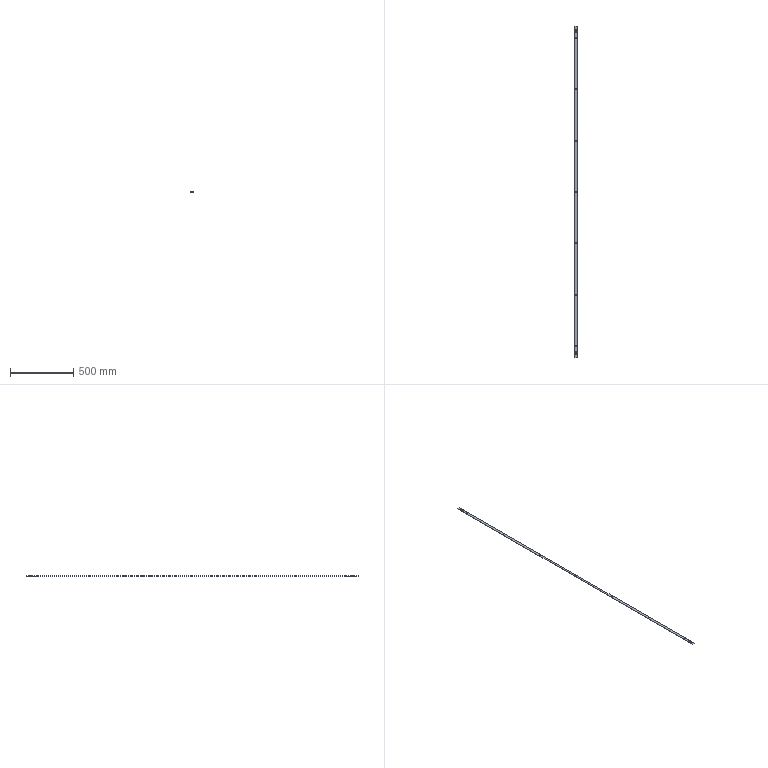Part | 1 solid | 36 faces | box 20 x 2616 x 1.5 mm | volume 77453 mm3 | cylinder 22 | plane 14 | commonest cylinder face diameters 6.2 x14 4 x8
STEP:
#1=CARTESIAN_POINT('',(-3.1,-1213.,-1.5));
#2=VERTEX_POINT('',#1);
#3=CARTESIAN_POINT('',(3.1,-1213.,-1.5));
#4=VERTEX_POINT('',#3);
#5=CARTESIAN_POINT('',(0.,-1213.,-1.5));
#6=DIRECTION('',(0.,0.,1.));
#7=DIRECTION('',(1.,0.,0.));
#8=AXIS2_PLACEMENT_3D('',#5,#6,#7);
#9=CIRCLE('',#8,3.1);
#10=EDGE_CURVE('',#2,#4,#9,.T.);
#11=ORIENTED_EDGE('',*,*,#10,.F.);
#12=CARTESIAN_POINT('',(-3.1,-1213.,0.));
#13=VERTEX_POINT('',#12);
#14=CARTESIAN_POINT('',(-3.1,-1213.,-10.));
#15=DIRECTION('',(0.,0.,1.));
#16=VECTOR('',#15,1000.);
#17=LINE('',#14,#16);
#18=EDGE_CURVE('',#2,#13,#17,.T.);
#19=ORIENTED_EDGE('',*,*,#18,.T.);
#20=CARTESIAN_POINT('',(3.1,-1213.,0.));
#21=VERTEX_POINT('',#20);
#22=CARTESIAN_POINT('',(0.,-1213.,0.));
#23=DIRECTION('',(0.,0.,1.));
#24=DIRECTION('',(-1.,0.,0.));
#25=AXIS2_PLACEMENT_3D('',#22,#23,#24);
#26=CIRCLE('',#25,3.1);
#27=EDGE_CURVE('',#13,#21,#26,.T.);
#28=ORIENTED_EDGE('',*,*,#27,.T.);
#29=CARTESIAN_POINT('',(3.1,-1213.,-10.));
#30=DIRECTION('',(0.,0.,1.));
#31=VECTOR('',#30,1000.);
#32=LINE('',#29,#31);
#33=EDGE_CURVE('',#4,#21,#32,.T.);
#34=ORIENTED_EDGE('',*,*,#33,.F.);
#35=EDGE_LOOP('',(#11,#19,#28,#34));
#36=FACE_OUTER_BOUND('',#35,.T.);
#37=CARTESIAN_POINT('',(0.,-1213.,-10.));
#38=DIRECTION('',(0.,0.,1.));
#39=DIRECTION('',(1.,0.,0.));
#40=AXIS2_PLACEMENT_3D('',#37,#38,#39);
#41=CYLINDRICAL_SURFACE('',#40,3.1);
#42=ADVANCED_FACE('',(#36),#41,.F.);
#43=CARTESIAN_POINT('',(-3.1,-808.667,-1.5));
#44=VERTEX_POINT('',#43);
#45=CARTESIAN_POINT('',(3.1,-808.667,-1.5));
#46=VERTEX_POINT('',#45);
#47=CARTESIAN_POINT('',(0.,-808.667,-1.5));
#48=DIRECTION('',(0.,0.,1.));
#49=DIRECTION('',(1.,0.,0.));
#50=AXIS2_PLACEMENT_3D('',#47,#48,#49);
#51=CIRCLE('',#50,3.1);
#52=EDGE_CURVE('',#44,#46,#51,.T.);
#53=ORIENTED_EDGE('',*,*,#52,.F.);
#54=CARTESIAN_POINT('',(-3.1,-808.667,0.));
#55=VERTEX_POINT('',#54);
#56=CARTESIAN_POINT('',(-3.1,-808.667,-10.));
#57=DIRECTION('',(0.,0.,1.));
#58=VECTOR('',#57,1000.);
#59=LINE('',#56,#58);
#60=EDGE_CURVE('',#44,#55,#59,.T.);
#61=ORIENTED_EDGE('',*,*,#60,.T.);
#62=CARTESIAN_POINT('',(3.1,-808.667,0.));
#63=VERTEX_POINT('',#62);
#64=CARTESIAN_POINT('',(0.,-808.667,0.));
#65=DIRECTION('',(0.,0.,1.));
#66=DIRECTION('',(-1.,0.,0.));
#67=AXIS2_PLACEMENT_3D('',#64,#65,#66);
#68=CIRCLE('',#67,3.1);
#69=EDGE_CURVE('',#55,#63,#68,.T.);
#70=ORIENTED_EDGE('',*,*,#69,.T.);
#71=CARTESIAN_POINT('',(3.1,-808.667,-10.));
#72=DIRECTION('',(0.,0.,1.));
#73=VECTOR('',#72,1000.);
#74=LINE('',#71,#73);
#75=EDGE_CURVE('',#46,#63,#74,.T.);
#76=ORIENTED_EDGE('',*,*,#75,.F.);
#77=EDGE_LOOP('',(#53,#61,#70,#76));
#78=FACE_OUTER_BOUND('',#77,.T.);
#79=CARTESIAN_POINT('',(0.,-808.667,-10.));
#80=DIRECTION('',(0.,0.,1.));
#81=DIRECTION('',(1.,0.,0.));
#82=AXIS2_PLACEMENT_3D('',#79,#80,#81);
#83=CYLINDRICAL_SURFACE('',#82,3.1);
#84=ADVANCED_FACE('',(#78),#83,.F.);
#85=CARTESIAN_POINT('',(-3.1,404.333,-1.5));
#86=VERTEX_POINT('',#85);
#87=CARTESIAN_POINT('',(3.1,404.333,-1.5));
#88=VERTEX_POINT('',#87);
#89=CARTESIAN_POINT('',(0.,404.333,-1.5));
#90=DIRECTION('',(0.,0.,1.));
#91=DIRECTION('',(1.,0.,0.));
#92=AXIS2_PLACEMENT_3D('',#89,#90,#91);
#93=CIRCLE('',#92,3.1);
#94=EDGE_CURVE('',#86,#88,#93,.T.);
#95=ORIENTED_EDGE('',*,*,#94,.F.);
#96=CARTESIAN_POINT('',(-3.1,404.333,0.));
#97=VERTEX_POINT('',#96);
#98=CARTESIAN_POINT('',(-3.1,404.333,-10.));
#99=DIRECTION('',(0.,0.,1.));
#100=VECTOR('',#99,1000.);
#101=LINE('',#98,#100);
#102=EDGE_CURVE('',#86,#97,#101,.T.);
#103=ORIENTED_EDGE('',*,*,#102,.T.);
#104=CARTESIAN_POINT('',(3.1,404.333,0.));
#105=VERTEX_POINT('',#104);
#106=CARTESIAN_POINT('',(0.,404.333,0.));
#107=DIRECTION('',(0.,0.,1.));
#108=DIRECTION('',(1.,0.,0.));
#109=AXIS2_PLACEMENT_3D('',#106,#107,#108);
#110=CIRCLE('',#109,3.1);
#111=EDGE_CURVE('',#97,#105,#110,.T.);
#112=ORIENTED_EDGE('',*,*,#111,.T.);
#113=CARTESIAN_POINT('',(3.1,404.333,-10.));
#114=DIRECTION('',(0.,0.,1.));
#115=VECTOR('',#114,1000.);
#116=LINE('',#113,#115);
#117=EDGE_CURVE('',#88,#105,#116,.T.);
#118=ORIENTED_EDGE('',*,*,#117,.F.);
#119=EDGE_LOOP('',(#95,#103,#112,#118));
#120=FACE_OUTER_BOUND('',#119,.T.);
#121=CARTESIAN_POINT('',(0.,404.333,-10.));
#122=DIRECTION('',(0.,0.,1.));
#123=DIRECTION('',(1.,0.,0.));
#124=AXIS2_PLACEMENT_3D('',#121,#122,#123);
#125=CYLINDRICAL_SURFACE('',#124,3.1);
#126=ADVANCED_FACE('',(#120),#125,.F.);
#127=CARTESIAN_POINT('',(-3.1,808.667,-1.5));
#128=VERTEX_POINT('',#127);
#129=CARTESIAN_POINT('',(3.1,808.667,-1.5));
#130=VERTEX_POINT('',#129);
#131=CARTESIAN_POINT('',(0.,808.667,-1.5));
#132=DIRECTION('',(0.,0.,1.));
#133=DIRECTION('',(1.,0.,0.));
#134=AXIS2_PLACEMENT_3D('',#131,#132,#133);
#135=CIRCLE('',#134,3.1);
#136=EDGE_CURVE('',#128,#130,#135,.T.);
#137=ORIENTED_EDGE('',*,*,#136,.F.);
#138=CARTESIAN_POINT('',(-3.1,808.667,0.));
#139=VERTEX_POINT('',#138);
#140=CARTESIAN_POINT('',(-3.1,808.667,-10.));
#141=DIRECTION('',(0.,0.,1.));
#142=VECTOR('',#141,1000.);
#143=LINE('',#140,#142);
#144=EDGE_CURVE('',#128,#139,#143,.T.);
#145=ORIENTED_EDGE('',*,*,#144,.T.);
#146=CARTESIAN_POINT('',(3.1,808.667,0.));
#147=VERTEX_POINT('',#146);
#148=CARTESIAN_POINT('',(0.,808.667,0.));
#149=DIRECTION('',(0.,0.,1.));
#150=DIRECTION('',(1.,0.,0.));
#151=AXIS2_PLACEMENT_3D('',#148,#149,#150);
#152=CIRCLE('',#151,3.1);
#153=EDGE_CURVE('',#139,#147,#152,.T.);
#154=ORIENTED_EDGE('',*,*,#153,.T.);
#155=CARTESIAN_POINT('',(3.1,808.667,-10.));
#156=DIRECTION('',(0.,0.,1.));
#157=VECTOR('',#156,1000.);
#158=LINE('',#155,#157);
#159=EDGE_CURVE('',#130,#147,#158,.T.);
#160=ORIENTED_EDGE('',*,*,#159,.F.);
#161=EDGE_LOOP('',(#137,#145,#154,#160));
#162=FACE_OUTER_BOUND('',#161,.T.);
#163=CARTESIAN_POINT('',(0.,808.667,-10.));
#164=DIRECTION('',(0.,0.,1.));
#165=DIRECTION('',(1.,0.,0.));
#166=AXIS2_PLACEMENT_3D('',#163,#164,#165);
#167=CYLINDRICAL_SURFACE('',#166,3.1);
#168=ADVANCED_FACE('',(#162),#167,.F.);
#169=CARTESIAN_POINT('',(-3.1,1213.,-1.5));
#170=VERTEX_POINT('',#169);
#171=CARTESIAN_POINT('',(3.1,1213.,-1.5));
#172=VERTEX_POINT('',#171);
#173=CARTESIAN_POINT('',(0.,1213.,-1.5));
#174=DIRECTION('',(0.,0.,1.));
#175=DIRECTION('',(1.,0.,0.));
#176=AXIS2_PLACEMENT_3D('',#173,#174,#175);
#177=CIRCLE('',#176,3.1);
#178=EDGE_CURVE('',#170,#172,#177,.T.);
#179=ORIENTED_EDGE('',*,*,#178,.F.);
#180=CARTESIAN_POINT('',(-3.1,1213.,0.));
#181=VERTEX_POINT('',#180);
#182=CARTESIAN_POINT('',(-3.1,1213.,-10.));
#183=DIRECTION('',(0.,0.,1.));
#184=VECTOR('',#183,1000.);
#185=LINE('',#182,#184);
#186=EDGE_CURVE('',#170,#181,#185,.T.);
#187=ORIENTED_EDGE('',*,*,#186,.T.);
#188=CARTESIAN_POINT('',(3.1,1213.,0.));
#189=VERTEX_POINT('',#188);
#190=CARTESIAN_POINT('',(0.,1213.,0.));
#191=DIRECTION('',(0.,0.,1.));
#192=DIRECTION('',(1.,0.,0.));
#193=AXIS2_PLACEMENT_3D('',#190,#191,#192);
#194=CIRCLE('',#193,3.1);
#195=EDGE_CURVE('',#181,#189,#194,.T.);
#196=ORIENTED_EDGE('',*,*,#195,.T.);
#197=CARTESIAN_POINT('',(3.1,1213.,-10.));
#198=DIRECTION('',(0.,0.,1.));
#199=VECTOR('',#198,1000.);
#200=LINE('',#197,#199);
#201=EDGE_CURVE('',#172,#189,#200,.T.);
#202=ORIENTED_EDGE('',*,*,#201,.F.);
#203=EDGE_LOOP('',(#179,#187,#196,#202));
#204=FACE_OUTER_BOUND('',#203,.T.);
#205=CARTESIAN_POINT('',(0.,1213.,-10.));
#206=DIRECTION('',(0.,0.,1.));
#207=DIRECTION('',(1.,0.,0.));
#208=AXIS2_PLACEMENT_3D('',#205,#206,#207);
#209=CYLINDRICAL_SURFACE('',#208,3.1);
#210=ADVANCED_FACE('',(#204),#209,.F.);
#211=CARTESIAN_POINT('',(-3.1,-404.333,-1.5));
#212=VERTEX_POINT('',#211);
#213=CARTESIAN_POINT('',(3.1,-404.333,-1.5));
#214=VERTEX_POINT('',#213);
#215=CARTESIAN_POINT('',(0.,-404.333,-1.5));
#216=DIRECTION('',(0.,0.,1.));
#217=DIRECTION('',(1.,0.,0.));
#218=AXIS2_PLACEMENT_3D('',#215,#216,#217);
#219=CIRCLE('',#218,3.1);
#220=EDGE_CURVE('',#212,#214,#219,.T.);
#221=ORIENTED_EDGE('',*,*,#220,.F.);
#222=CARTESIAN_POINT('',(-3.1,-404.333,0.));
#223=VERTEX_POINT('',#222);
#224=CARTESIAN_POINT('',(-3.1,-404.333,-10.));
#225=DIRECTION('',(0.,0.,1.));
#226=VECTOR('',#225,1000.);
#227=LINE('',#224,#226);
#228=EDGE_CURVE('',#212,#223,#227,.T.);
#229=ORIENTED_EDGE('',*,*,#228,.T.);
#230=CARTESIAN_POINT('',(3.1,-404.333,0.));
#231=VERTEX_POINT('',#230);
#232=CARTESIAN_POINT('',(0.,-404.333,0.));
#233=DIRECTION('',(0.,0.,1.));
#234=DIRECTION('',(-1.,0.,0.));
#235=AXIS2_PLACEMENT_3D('',#232,#233,#234);
#236=CIRCLE('',#235,3.1);
#237=EDGE_CURVE('',#223,#231,#236,.T.);
#238=ORIENTED_EDGE('',*,*,#237,.T.);
#239=CARTESIAN_POINT('',(3.1,-404.333,-10.));
#240=DIRECTION('',(0.,0.,1.));
#241=VECTOR('',#240,1000.);
#242=LINE('',#239,#241);
#243=EDGE_CURVE('',#214,#231,#242,.T.);
#244=ORIENTED_EDGE('',*,*,#243,.F.);
#245=EDGE_LOOP('',(#221,#229,#238,#244));
#246=FACE_OUTER_BOUND('',#245,.T.);
#247=CARTESIAN_POINT('',(0.,-404.333,-10.));
#248=DIRECTION('',(0.,0.,1.));
#249=DIRECTION('',(1.,0.,0.));
#250=AXIS2_PLACEMENT_3D('',#247,#248,#249);
#251=CYLINDRICAL_SURFACE('',#250,3.1);
#252=ADVANCED_FACE('',(#246),#251,.F.);
#253=CARTESIAN_POINT('',(-3.1,0.,-1.5));
#254=VERTEX_POINT('',#253);
#255=CARTESIAN_POINT('',(3.1,0.,-1.5));
#256=VERTEX_POINT('',#255);
#257=CARTESIAN_POINT('',(0.,0.,-1.5));
#258=DIRECTION('',(0.,0.,1.));
#259=DIRECTION('',(1.,0.,0.));
#260=AXIS2_PLACEMENT_3D('',#257,#258,#259);
#261=CIRCLE('',#260,3.1);
#262=EDGE_CURVE('',#254,#256,#261,.T.);
#263=ORIENTED_EDGE('',*,*,#262,.F.);
#264=CARTESIAN_POINT('',(-3.1,0.,0.));
#265=VERTEX_POINT('',#264);
#266=CARTESIAN_POINT('',(-3.1,0.,-10.));
#267=DIRECTION('',(0.,0.,1.));
#268=VECTOR('',#267,1000.);
#269=LINE('',#266,#268);
#270=EDGE_CURVE('',#254,#265,#269,.T.);
#271=ORIENTED_EDGE('',*,*,#270,.T.);
#272=CARTESIAN_POINT('',(3.1,0.,0.));
#273=VERTEX_POINT('',#272);
#274=CARTESIAN_POINT('',(0.,0.,0.));
#275=DIRECTION('',(0.,0.,1.));
#276=DIRECTION('',(1.,0.,0.));
#277=AXIS2_PLACEMENT_3D('',#274,#275,#276);
#278=CIRCLE('',#277,3.1);
#279=EDGE_CURVE('',#265,#273,#278,.T.);
#280=ORIENTED_EDGE('',*,*,#279,.T.);
#281=CARTESIAN_POINT('',(3.1,0.,-10.));
#282=DIRECTION('',(0.,0.,1.));
#283=VECTOR('',#282,1000.);
#284=LINE('',#281,#283);
#285=EDGE_CURVE('',#256,#273,#284,.T.);
#286=ORIENTED_EDGE('',*,*,#285,.F.);
#287=EDGE_LOOP('',(#263,#271,#280,#286));
#288=FACE_OUTER_BOUND('',#287,.T.);
#289=CARTESIAN_POINT('',(0.,0.,-10.));
#290=DIRECTION('',(0.,0.,1.));
#291=DIRECTION('',(1.,0.,0.));
#292=AXIS2_PLACEMENT_3D('',#289,#290,#291);
#293=CYLINDRICAL_SURFACE('',#292,3.1);
#294=ADVANCED_FACE('',(#288),#293,.F.);
#295=CARTESIAN_POINT('',(10.,-1308.,0.));
#296=VERTEX_POINT('',#295);
#297=CARTESIAN_POINT('',(10.,1308.,0.));
#298=VERTEX_POINT('',#297);
#299=CARTESIAN_POINT('',(10.,1308.,0.));
#300=DIRECTION('',(0.,1.,0.));
#301=VECTOR('',#300,1000.);
#302=LINE('',#299,#301);
#303=EDGE_CURVE('',#296,#298,#302,.T.);
#304=ORIENTED_EDGE('',*,*,#303,.F.);
#305=CARTESIAN_POINT('',(10.,-1308.,-1.5));
#306=VERTEX_POINT('',#305);
#307=CARTESIAN_POINT('',(10.,-1308.,-1.5));
#308=DIRECTION('',(0.,0.,1.));
#309=VECTOR('',#308,1000.);
#310=LINE('',#307,#309);
#311=EDGE_CURVE('',#306,#296,#310,.T.);
#312=ORIENTED_EDGE('',*,*,#311,.F.);
#313=CARTESIAN_POINT('',(10.,1308.,-1.5));
#314=VERTEX_POINT('',#313);
#315=CARTESIAN_POINT('',(10.,1308.,-1.5));
#316=DIRECTION('',(0.,1.,0.));
#317=VECTOR('',#316,1000.);
#318=LINE('',#315,#317);
#319=EDGE_CURVE('',#306,#314,#318,.T.);
#320=ORIENTED_EDGE('',*,*,#319,.T.);
#321=CARTESIAN_POINT('',(10.,1308.,-1.5));
#322=DIRECTION('',(0.,0.,1.));
#323=VECTOR('',#322,1000.);
#324=LINE('',#321,#323);
#325=EDGE_CURVE('',#314,#298,#324,.T.);
#326=ORIENTED_EDGE('',*,*,#325,.T.);
#327=EDGE_LOOP('',(#304,#312,#320,#326));
#328=FACE_OUTER_BOUND('',#327,.T.);
#329=CARTESIAN_POINT('',(10.,1308.,-1.5));
#330=DIRECTION('',(1.,0.,0.));
#331=DIRECTION('',(0.,1.,0.));
#332=AXIS2_PLACEMENT_3D('',#329,#330,#331);
#333=PLANE('',#332);
#334=ADVANCED_FACE('',(#328),#333,.T.);
#335=CARTESIAN_POINT('',(-10.,-1308.,0.));
#336=VERTEX_POINT('',#335);
#337=CARTESIAN_POINT('',(-10.,-1308.,0.));
#338=DIRECTION('',(1.,0.,0.));
#339=VECTOR('',#338,1000.);
#340=LINE('',#337,#339);
#341=EDGE_CURVE('',#336,#296,#340,.T.);
#342=ORIENTED_EDGE('',*,*,#341,.F.);
#343=CARTESIAN_POINT('',(-10.,-1308.,-1.5));
#344=VERTEX_POINT('',#343);
#345=CARTESIAN_POINT('',(-10.,-1308.,-1.5));
#346=DIRECTION('',(0.,0.,1.));
#347=VECTOR('',#346,1000.);
#348=LINE('',#345,#347);
#349=EDGE_CURVE('',#344,#336,#348,.T.);
#350=ORIENTED_EDGE('',*,*,#349,.F.);
#351=CARTESIAN_POINT('',(-10.,-1308.,-1.5));
#352=DIRECTION('',(1.,0.,0.));
#353=VECTOR('',#352,1000.);
#354=LINE('',#351,#353);
#355=EDGE_CURVE('',#344,#306,#354,.T.);
#356=ORIENTED_EDGE('',*,*,#355,.T.);
#357=ORIENTED_EDGE('',*,*,#311,.T.);
#358=EDGE_LOOP('',(#342,#350,#356,#357));
#359=FACE_OUTER_BOUND('',#358,.T.);
#360=CARTESIAN_POINT('',(-10.,-1308.,-1.5));
#361=DIRECTION('',(0.,-1.,0.));
#362=DIRECTION('',(0.,0.,-1.));
#363=AXIS2_PLACEMENT_3D('',#360,#361,#362);
#364=PLANE('',#363);
#365=ADVANCED_FACE('',(#359),#364,.T.);
#366=CARTESIAN_POINT('',(-10.,1308.,0.));
#367=VERTEX_POINT('',#366);
#368=CARTESIAN_POINT('',(-10.,1308.,0.));
#369=DIRECTION('',(0.,-1.,0.));
#370=VECTOR('',#369,1000.);
#371=LINE('',#368,#370);
#372=EDGE_CURVE('',#367,#336,#371,.T.);
#373=ORIENTED_EDGE('',*,*,#372,.F.);
#374=CARTESIAN_POINT('',(-10.,1308.,-1.5));
#375=VERTEX_POINT('',#374);
#376=CARTESIAN_POINT('',(-10.,1308.,-1.5));
#377=DIRECTION('',(0.,0.,1.));
#378=VECTOR('',#377,1000.);
#379=LINE('',#376,#378);
#380=EDGE_CURVE('',#375,#367,#379,.T.);
#381=ORIENTED_EDGE('',*,*,#380,.F.);
#382=CARTESIAN_POINT('',(-10.,1308.,-1.5));
#383=DIRECTION('',(0.,-1.,0.));
#384=VECTOR('',#383,1000.);
#385=LINE('',#382,#384);
#386=EDGE_CURVE('',#375,#344,#385,.T.);
#387=ORIENTED_EDGE('',*,*,#386,.T.);
#388=ORIENTED_EDGE('',*,*,#349,.T.);
#389=EDGE_LOOP('',(#373,#381,#387,#388));
#390=FACE_OUTER_BOUND('',#389,.T.);
#391=CARTESIAN_POINT('',(-10.,1308.,-1.5));
#392=DIRECTION('',(-1.,0.,0.));
#393=DIRECTION('',(0.,-1.,0.));
#394=AXIS2_PLACEMENT_3D('',#391,#392,#393);
#395=PLANE('',#394);
#396=ADVANCED_FACE('',(#390),#395,.T.);
#397=CARTESIAN_POINT('',(-10.,1308.,0.));
#398=DIRECTION('',(-1.,0.,0.));
#399=VECTOR('',#398,1000.);
#400=LINE('',#397,#399);
#401=EDGE_CURVE('',#298,#367,#400,.T.);
#402=ORIENTED_EDGE('',*,*,#401,.F.);
#403=ORIENTED_EDGE('',*,*,#325,.F.);
#404=CARTESIAN_POINT('',(-10.,1308.,-1.5));
#405=DIRECTION('',(-1.,0.,0.));
#406=VECTOR('',#405,1000.);
#407=LINE('',#404,#406);
#408=EDGE_CURVE('',#314,#375,#407,.T.);
#409=ORIENTED_EDGE('',*,*,#408,.T.);
#410=ORIENTED_EDGE('',*,*,#380,.T.);
#411=EDGE_LOOP('',(#402,#403,#409,#410));
#412=FACE_OUTER_BOUND('',#411,.T.);
#413=CARTESIAN_POINT('',(-10.,1308.,-1.5));
#414=DIRECTION('',(0.,1.,0.));
#415=DIRECTION('',(0.,0.,1.));
#416=AXIS2_PLACEMENT_3D('',#413,#414,#415);
#417=PLANE('',#416);
#418=ADVANCED_FACE('',(#412),#417,.T.);
#419=CARTESIAN_POINT('',(-4.,-1255.,-1.5));
#420=VERTEX_POINT('',#419);
#421=CARTESIAN_POINT('',(-4.,-1281.,-1.5));
#422=VERTEX_POINT('',#421);
#423=CARTESIAN_POINT('',(-4.,0.,-1.5));
#424=DIRECTION('',(0.,-1.,0.));
#425=VECTOR('',#424,1000.);
#426=LINE('',#423,#425);
#427=EDGE_CURVE('',#420,#422,#426,.T.);
#428=ORIENTED_EDGE('',*,*,#427,.T.);
#429=CARTESIAN_POINT('',(-2.,-1283.,-1.5));
#430=VERTEX_POINT('',#429);
#431=CARTESIAN_POINT('',(-2.,-1281.,-1.5));
#432=DIRECTION('',(0.,0.,1.));
#433=DIRECTION('',(1.,0.,0.));
#434=AXIS2_PLACEMENT_3D('',#431,#432,#433);
#435=CIRCLE('',#434,2.);
#436=EDGE_CURVE('',#422,#430,#435,.T.);
#437=ORIENTED_EDGE('',*,*,#436,.T.);
#438=CARTESIAN_POINT('',(2.,-1283.,-1.5));
#439=VERTEX_POINT('',#438);
#440=CARTESIAN_POINT('',(0.,-1283.,-1.5));
#441=DIRECTION('',(1.,0.,0.));
#442=VECTOR('',#441,1000.);
#443=LINE('',#440,#442);
#444=EDGE_CURVE('',#430,#439,#443,.T.);
#445=ORIENTED_EDGE('',*,*,#444,.T.);
#446=CARTESIAN_POINT('',(4.,-1281.,-1.5));
#447=VERTEX_POINT('',#446);
#448=CARTESIAN_POINT('',(2.,-1281.,-1.5));
#449=DIRECTION('',(0.,0.,1.));
#450=DIRECTION('',(1.,0.,0.));
#451=AXIS2_PLACEMENT_3D('',#448,#449,#450);
#452=CIRCLE('',#451,2.);
#453=EDGE_CURVE('',#439,#447,#452,.T.);
#454=ORIENTED_EDGE('',*,*,#453,.T.);
#455=CARTESIAN_POINT('',(4.,-1255.,-1.5));
#456=VERTEX_POINT('',#455);
#457=CARTESIAN_POINT('',(4.,0.,-1.5));
#458=DIRECTION('',(0.,1.,0.));
#459=VECTOR('',#458,1000.);
#460=LINE('',#457,#459);
#461=EDGE_CURVE('',#447,#456,#460,.T.);
#462=ORIENTED_EDGE('',*,*,#461,.T.);
#463=CARTESIAN_POINT('',(2.,-1253.,-1.5));
#464=VERTEX_POINT('',#463);
#465=CARTESIAN_POINT('',(2.,-1255.,-1.5));
#466=DIRECTION('',(0.,0.,1.));
#467=DIRECTION('',(1.,0.,0.));
#468=AXIS2_PLACEMENT_3D('',#465,#466,#467);
#469=CIRCLE('',#468,2.);
#470=EDGE_CURVE('',#456,#464,#469,.T.);
#471=ORIENTED_EDGE('',*,*,#470,.T.);
#472=CARTESIAN_POINT('',(-2.,-1253.,-1.5));
#473=VERTEX_POINT('',#472);
#474=CARTESIAN_POINT('',(0.,-1253.,-1.5));
#475=DIRECTION('',(-1.,0.,0.));
#476=VECTOR('',#475,1000.);
#477=LINE('',#474,#476);
#478=EDGE_CURVE('',#464,#473,#477,.T.);
#479=ORIENTED_EDGE('',*,*,#478,.T.);
#480=CARTESIAN_POINT('',(-2.,-1255.,-1.5));
#481=DIRECTION('',(0.,0.,1.));
#482=DIRECTION('',(1.,0.,0.));
#483=AXIS2_PLACEMENT_3D('',#480,#481,#482);
#484=CIRCLE('',#483,2.);
#485=EDGE_CURVE('',#473,#420,#484,.T.);
#486=ORIENTED_EDGE('',*,*,#485,.T.);
#487=EDGE_LOOP('',(#428,#437,#445,#454,#462,#471,#479,#486));
#488=FACE_BOUND('',#487,.T.);
#489=CARTESIAN_POINT('',(4.,1255.,-1.5));
#490=VERTEX_POINT('',#489);
#491=CARTESIAN_POINT('',(4.,1281.,-1.5));
#492=VERTEX_POINT('',#491);
#493=CARTESIAN_POINT('',(4.,0.,-1.5));
#494=DIRECTION('',(0.,1.,0.));
#495=VECTOR('',#494,1000.);
#496=LINE('',#493,#495);
#497=EDGE_CURVE('',#490,#492,#496,.T.);
#498=ORIENTED_EDGE('',*,*,#497,.T.);
#499=CARTESIAN_POINT('',(2.,1283.,-1.5));
#500=VERTEX_POINT('',#499);
#501=CARTESIAN_POINT('',(2.,1281.,-1.5));
#502=DIRECTION('',(0.,0.,1.));
#503=DIRECTION('',(1.,0.,0.));
#504=AXIS2_PLACEMENT_3D('',#501,#502,#503);
#505=CIRCLE('',#504,2.);
#506=EDGE_CURVE('',#492,#500,#505,.T.);
#507=ORIENTED_EDGE('',*,*,#506,.T.);
#508=CARTESIAN_POINT('',(-2.,1283.,-1.5));
#509=VERTEX_POINT('',#508);
#510=CARTESIAN_POINT('',(0.,1283.,-1.5));
#511=DIRECTION('',(-1.,0.,0.));
#512=VECTOR('',#511,1000.);
#513=LINE('',#510,#512);
#514=EDGE_CURVE('',#500,#509,#513,.T.);
#515=ORIENTED_EDGE('',*,*,#514,.T.);
#516=CARTESIAN_POINT('',(-4.,1281.,-1.5));
#517=VERTEX_POINT('',#516);
#518=CARTESIAN_POINT('',(-2.,1281.,-1.5));
#519=DIRECTION('',(0.,0.,1.));
#520=DIRECTION('',(1.,0.,0.));
#521=AXIS2_PLACEMENT_3D('',#518,#519,#520);
#522=CIRCLE('',#521,2.);
#523=EDGE_CURVE('',#509,#517,#522,.T.);
#524=ORIENTED_EDGE('',*,*,#523,.T.);
#525=CARTESIAN_POINT('',(-4.,1255.,-1.5));
#526=VERTEX_POINT('',#525);
#527=CARTESIAN_POINT('',(-4.,0.,-1.5));
#528=DIRECTION('',(0.,-1.,0.));
#529=VECTOR('',#528,1000.);
#530=LINE('',#527,#529);
#531=EDGE_CURVE('',#517,#526,#530,.T.);
#532=ORIENTED_EDGE('',*,*,#531,.T.);
#533=CARTESIAN_POINT('',(-2.,1253.,-1.5));
#534=VERTEX_POINT('',#533);
#535=CARTESIAN_POINT('',(-2.,1255.,-1.5));
#536=DIRECTION('',(0.,0.,1.));
#537=DIRECTION('',(1.,0.,0.));
#538=AXIS2_PLACEMENT_3D('',#535,#536,#537);
#539=CIRCLE('',#538,2.);
#540=EDGE_CURVE('',#526,#534,#539,.T.);
#541=ORIENTED_EDGE('',*,*,#540,.T.);
#542=CARTESIAN_POINT('',(2.,1253.,-1.5));
#543=VERTEX_POINT('',#542);
#544=CARTESIAN_POINT('',(0.,1253.,-1.5));
#545=DIRECTION('',(1.,0.,0.));
#546=VECTOR('',#545,1000.);
#547=LINE('',#544,#546);
#548=EDGE_CURVE('',#534,#543,#547,.T.);
#549=ORIENTED_EDGE('',*,*,#548,.T.);
#550=CARTESIAN_POINT('',(2.,1255.,-1.5));
#551=DIRECTION('',(0.,0.,1.));
#552=DIRECTION('',(1.,0.,0.));
#553=AXIS2_PLACEMENT_3D('',#550,#551,#552);
#554=CIRCLE('',#553,2.);
#555=EDGE_CURVE('',#543,#490,#554,.T.);
#556=ORIENTED_EDGE('',*,*,#555,.T.);
#557=EDGE_LOOP('',(#498,#507,#515,#524,#532,#541,#549,#556));
#558=FACE_BOUND('',#557,.T.);
#559=CARTESIAN_POINT('',(0.,-1213.,-1.5));
#560=DIRECTION('',(0.,0.,1.));
#561=DIRECTION('',(1.,0.,0.));
#562=AXIS2_PLACEMENT_3D('',#559,#560,#561);
#563=CIRCLE('',#562,3.1);
#564=EDGE_CURVE('',#4,#2,#563,.T.);
#565=ORIENTED_EDGE('',*,*,#564,.T.);
#566=ORIENTED_EDGE('',*,*,#10,.T.);
#567=EDGE_LOOP('',(#565,#566));
#568=FACE_BOUND('',#567,.T.);
#569=CARTESIAN_POINT('',(0.,-808.667,-1.5));
#570=DIRECTION('',(0.,0.,1.));
#571=DIRECTION('',(1.,0.,0.));
#572=AXIS2_PLACEMENT_3D('',#569,#570,#571);
#573=CIRCLE('',#572,3.1);
#574=EDGE_CURVE('',#46,#44,#573,.T.);
#575=ORIENTED_EDGE('',*,*,#574,.T.);
#576=ORIENTED_EDGE('',*,*,#52,.T.);
#577=EDGE_LOOP('',(#575,#576));
#578=FACE_BOUND('',#577,.T.);
#579=CARTESIAN_POINT('',(0.,404.333,-1.5));
#580=DIRECTION('',(0.,0.,1.));
#581=DIRECTION('',(1.,0.,0.));
#582=AXIS2_PLACEMENT_3D('',#579,#580,#581);
#583=CIRCLE('',#582,3.1);
#584=EDGE_CURVE('',#88,#86,#583,.T.);
#585=ORIENTED_EDGE('',*,*,#584,.T.);
#586=ORIENTED_EDGE('',*,*,#94,.T.);
#587=EDGE_LOOP('',(#585,#586));
#588=FACE_BOUND('',#587,.T.);
#589=CARTESIAN_POINT('',(0.,808.667,-1.5));
#590=DIRECTION('',(0.,0.,1.));
#591=DIRECTION('',(1.,0.,0.));
#592=AXIS2_PLACEMENT_3D('',#589,#590,#591);
#593=CIRCLE('',#592,3.1);
#594=EDGE_CURVE('',#130,#128,#593,.T.);
#595=ORIENTED_EDGE('',*,*,#594,.T.);
#596=ORIENTED_EDGE('',*,*,#136,.T.);
#597=EDGE_LOOP('',(#595,#596));
#598=FACE_BOUND('',#597,.T.);
#599=CARTESIAN_POINT('',(0.,1213.,-1.5));
#600=DIRECTION('',(0.,0.,1.));
#601=DIRECTION('',(1.,0.,0.));
#602=AXIS2_PLACEMENT_3D('',#599,#600,#601);
#603=CIRCLE('',#602,3.1);
#604=EDGE_CURVE('',#172,#170,#603,.T.);
#605=ORIENTED_EDGE('',*,*,#604,.T.);
#606=ORIENTED_EDGE('',*,*,#178,.T.);
#607=EDGE_LOOP('',(#605,#606));
#608=FACE_BOUND('',#607,.T.);
#609=CARTESIAN_POINT('',(0.,-404.333,-1.5));
#610=DIRECTION('',(0.,0.,1.));
#611=DIRECTION('',(1.,0.,0.));
#612=AXIS2_PLACEMENT_3D('',#609,#610,#611);
#613=CIRCLE('',#612,3.1);
#614=EDGE_CURVE('',#214,#212,#613,.T.);
#615=ORIENTED_EDGE('',*,*,#614,.T.);
#616=ORIENTED_EDGE('',*,*,#220,.T.);
#617=EDGE_LOOP('',(#615,#616));
#618=FACE_BOUND('',#617,.T.);
#619=CARTESIAN_POINT('',(0.,0.,-1.5));
#620=DIRECTION('',(0.,0.,1.));
#621=DIRECTION('',(1.,0.,0.));
#622=AXIS2_PLACEMENT_3D('',#619,#620,#621);
#623=CIRCLE('',#622,3.1);
#624=EDGE_CURVE('',#256,#254,#623,.T.);
#625=ORIENTED_EDGE('',*,*,#624,.T.);
#626=ORIENTED_EDGE('',*,*,#262,.T.);
#627=EDGE_LOOP('',(#625,#626));
#628=FACE_BOUND('',#627,.T.);
#629=ORIENTED_EDGE('',*,*,#319,.F.);
#630=ORIENTED_EDGE('',*,*,#355,.F.);
#631=ORIENTED_EDGE('',*,*,#386,.F.);
#632=ORIENTED_EDGE('',*,*,#408,.F.);
#633=EDGE_LOOP('',(#629,#630,#631,#632));
#634=FACE_OUTER_BOUND('',#633,.T.);
#635=CARTESIAN_POINT('',(0.,0.,-1.5));
#636=DIRECTION('',(0.,0.,1.));
#637=DIRECTION('',(1.,0.,0.));
#638=AXIS2_PLACEMENT_3D('',#635,#636,#637);
#639=PLANE('',#638);
#640=ADVANCED_FACE('',(#488,#558,#568,#578,#588,#598,#608,#618,#628,#634),#639,.F.);
#641=CARTESIAN_POINT('',(4.,-1281.,0.));
#642=VERTEX_POINT('',#641);
#643=CARTESIAN_POINT('',(4.,-1255.,0.));
#644=VERTEX_POINT('',#643);
#645=CARTESIAN_POINT('',(4.,-1253.,0.));
#646=DIRECTION('',(0.,1.,0.));
#647=VECTOR('',#646,1000.);
#648=LINE('',#645,#647);
#649=EDGE_CURVE('',#642,#644,#648,.T.);
#650=ORIENTED_EDGE('',*,*,#649,.F.);
#651=CARTESIAN_POINT('',(2.,-1283.,0.));
#652=VERTEX_POINT('',#651);
#653=CARTESIAN_POINT('',(2.,-1281.,0.));
#654=DIRECTION('',(0.,0.,-1.));
#655=DIRECTION('',(1.,0.,0.));
#656=AXIS2_PLACEMENT_3D('',#653,#654,#655);
#657=CIRCLE('',#656,2.);
#658=EDGE_CURVE('',#642,#652,#657,.T.);
#659=ORIENTED_EDGE('',*,*,#658,.T.);
#660=CARTESIAN_POINT('',(-2.,-1283.,0.));
#661=VERTEX_POINT('',#660);
#662=CARTESIAN_POINT('',(-4.,-1283.,0.));
#663=DIRECTION('',(1.,0.,0.));
#664=VECTOR('',#663,1000.);
#665=LINE('',#662,#664);
#666=EDGE_CURVE('',#661,#652,#665,.T.);
#667=ORIENTED_EDGE('',*,*,#666,.F.);
#668=CARTESIAN_POINT('',(-4.,-1281.,0.));
#669=VERTEX_POINT('',#668);
#670=CARTESIAN_POINT('',(-2.,-1281.,0.));
#671=DIRECTION('',(0.,0.,-1.));
#672=DIRECTION('',(1.,0.,0.));
#673=AXIS2_PLACEMENT_3D('',#670,#671,#672);
#674=CIRCLE('',#673,2.);
#675=EDGE_CURVE('',#661,#669,#674,.T.);
#676=ORIENTED_EDGE('',*,*,#675,.T.);
#677=CARTESIAN_POINT('',(-4.,-1255.,0.));
#678=VERTEX_POINT('',#677);
#679=CARTESIAN_POINT('',(-4.,-1253.,0.));
#680=DIRECTION('',(0.,-1.,0.));
#681=VECTOR('',#680,1000.);
#682=LINE('',#679,#681);
#683=EDGE_CURVE('',#678,#669,#682,.T.);
#684=ORIENTED_EDGE('',*,*,#683,.F.);
#685=CARTESIAN_POINT('',(-2.,-1253.,0.));
#686=VERTEX_POINT('',#685);
#687=CARTESIAN_POINT('',(-2.,-1255.,0.));
#688=DIRECTION('',(0.,0.,-1.));
#689=DIRECTION('',(1.,0.,0.));
#690=AXIS2_PLACEMENT_3D('',#687,#688,#689);
#691=CIRCLE('',#690,2.);
#692=EDGE_CURVE('',#678,#686,#691,.T.);
#693=ORIENTED_EDGE('',*,*,#692,.T.);
#694=CARTESIAN_POINT('',(2.,-1253.,0.));
#695=VERTEX_POINT('',#694);
#696=CARTESIAN_POINT('',(-4.,-1253.,0.));
#697=DIRECTION('',(-1.,0.,0.));
#698=VECTOR('',#697,1000.);
#699=LINE('',#696,#698);
#700=EDGE_CURVE('',#695,#686,#699,.T.);
#701=ORIENTED_EDGE('',*,*,#700,.F.);
#702=CARTESIAN_POINT('',(2.,-1255.,0.));
#703=DIRECTION('',(0.,0.,-1.));
#704=DIRECTION('',(1.,0.,0.));
#705=AXIS2_PLACEMENT_3D('',#702,#703,#704);
#706=CIRCLE('',#705,2.);
#707=EDGE_CURVE('',#695,#644,#706,.T.);
#708=ORIENTED_EDGE('',*,*,#707,.T.);
#709=EDGE_LOOP('',(#650,#659,#667,#676,#684,#693,#701,#708));
#710=FACE_BOUND('',#709,.T.);
#711=CARTESIAN_POINT('',(-4.,1281.,0.));
#712=VERTEX_POINT('',#711);
#713=CARTESIAN_POINT('',(-4.,1255.,0.));
#714=VERTEX_POINT('',#713);
#715=CARTESIAN_POINT('',(-4.,1253.,0.));
#716=DIRECTION('',(0.,-1.,0.));
#717=VECTOR('',#716,1000.);
#718=LINE('',#715,#717);
#719=EDGE_CURVE('',#712,#714,#718,.T.);
#720=ORIENTED_EDGE('',*,*,#719,.F.);
#721=CARTESIAN_POINT('',(-2.,1283.,0.));
#722=VERTEX_POINT('',#721);
#723=CARTESIAN_POINT('',(-2.,1281.,0.));
#724=DIRECTION('',(0.,0.,-1.));
#725=DIRECTION('',(1.,0.,0.));
#726=AXIS2_PLACEMENT_3D('',#723,#724,#725);
#727=CIRCLE('',#726,2.);
#728=EDGE_CURVE('',#712,#722,#727,.T.);
#729=ORIENTED_EDGE('',*,*,#728,.T.);
#730=CARTESIAN_POINT('',(2.,1283.,0.));
#731=VERTEX_POINT('',#730);
#732=CARTESIAN_POINT('',(-4.,1283.,0.));
#733=DIRECTION('',(-1.,0.,0.));
#734=VECTOR('',#733,1000.);
#735=LINE('',#732,#734);
#736=EDGE_CURVE('',#731,#722,#735,.T.);
#737=ORIENTED_EDGE('',*,*,#736,.F.);
#738=CARTESIAN_POINT('',(4.,1281.,0.));
#739=VERTEX_POINT('',#738);
#740=CARTESIAN_POINT('',(2.,1281.,0.));
#741=DIRECTION('',(0.,0.,-1.));
#742=DIRECTION('',(1.,0.,0.));
#743=AXIS2_PLACEMENT_3D('',#740,#741,#742);
#744=CIRCLE('',#743,2.);
#745=EDGE_CURVE('',#731,#739,#744,.T.);
#746=ORIENTED_EDGE('',*,*,#745,.T.);
#747=CARTESIAN_POINT('',(4.,1255.,0.));
#748=VERTEX_POINT('',#747);
#749=CARTESIAN_POINT('',(4.,1253.,0.));
#750=DIRECTION('',(0.,1.,0.));
#751=VECTOR('',#750,1000.);
#752=LINE('',#749,#751);
#753=EDGE_CURVE('',#748,#739,#752,.T.);
#754=ORIENTED_EDGE('',*,*,#753,.F.);
#755=CARTESIAN_POINT('',(2.,1253.,0.));
#756=VERTEX_POINT('',#755);
#757=CARTESIAN_POINT('',(2.,1255.,0.));
#758=DIRECTION('',(0.,0.,-1.));
#759=DIRECTION('',(1.,0.,0.));
#760=AXIS2_PLACEMENT_3D('',#757,#758,#759);
#761=CIRCLE('',#760,2.);
#762=EDGE_CURVE('',#748,#756,#761,.T.);
#763=ORIENTED_EDGE('',*,*,#762,.T.);
#764=CARTESIAN_POINT('',(-2.,1253.,0.));
#765=VERTEX_POINT('',#764);
#766=CARTESIAN_POINT('',(-4.,1253.,0.));
#767=DIRECTION('',(1.,0.,0.));
#768=VECTOR('',#767,1000.);
#769=LINE('',#766,#768);
#770=EDGE_CURVE('',#765,#756,#769,.T.);
#771=ORIENTED_EDGE('',*,*,#770,.F.);
#772=CARTESIAN_POINT('',(-2.,1255.,0.));
#773=DIRECTION('',(0.,0.,-1.));
#774=DIRECTION('',(1.,0.,0.));
#775=AXIS2_PLACEMENT_3D('',#772,#773,#774);
#776=CIRCLE('',#775,2.);
#777=EDGE_CURVE('',#765,#714,#776,.T.);
#778=ORIENTED_EDGE('',*,*,#777,.T.);
#779=EDGE_LOOP('',(#720,#729,#737,#746,#754,#763,#771,#778));
#780=FACE_BOUND('',#779,.T.);
#781=CARTESIAN_POINT('',(0.,-1213.,0.));
#782=DIRECTION('',(0.,0.,1.));
#783=DIRECTION('',(-1.,0.,0.));
#784=AXIS2_PLACEMENT_3D('',#781,#782,#783);
#785=CIRCLE('',#784,3.1);
#786=EDGE_CURVE('',#21,#13,#785,.T.);
#787=ORIENTED_EDGE('',*,*,#786,.F.);
#788=ORIENTED_EDGE('',*,*,#27,.F.);
#789=EDGE_LOOP('',(#787,#788));
#790=FACE_BOUND('',#789,.T.);
#791=CARTESIAN_POINT('',(0.,-808.667,0.));
#792=DIRECTION('',(0.,0.,1.));
#793=DIRECTION('',(-1.,0.,0.));
#794=AXIS2_PLACEMENT_3D('',#791,#792,#793);
#795=CIRCLE('',#794,3.1);
#796=EDGE_CURVE('',#63,#55,#795,.T.);
#797=ORIENTED_EDGE('',*,*,#796,.F.);
#798=ORIENTED_EDGE('',*,*,#69,.F.);
#799=EDGE_LOOP('',(#797,#798));
#800=FACE_BOUND('',#799,.T.);
#801=CARTESIAN_POINT('',(0.,404.333,0.));
#802=DIRECTION('',(0.,0.,1.));
#803=DIRECTION('',(1.,0.,0.));
#804=AXIS2_PLACEMENT_3D('',#801,#802,#803);
#805=CIRCLE('',#804,3.1);
#806=EDGE_CURVE('',#105,#97,#805,.T.);
#807=ORIENTED_EDGE('',*,*,#806,.F.);
#808=ORIENTED_EDGE('',*,*,#111,.F.);
#809=EDGE_LOOP('',(#807,#808));
#810=FACE_BOUND('',#809,.T.);
#811=CARTESIAN_POINT('',(0.,808.667,0.));
#812=DIRECTION('',(0.,0.,1.));
#813=DIRECTION('',(1.,0.,0.));
#814=AXIS2_PLACEMENT_3D('',#811,#812,#813);
#815=CIRCLE('',#814,3.1);
#816=EDGE_CURVE('',#147,#139,#815,.T.);
#817=ORIENTED_EDGE('',*,*,#816,.F.);
#818=ORIENTED_EDGE('',*,*,#153,.F.);
#819=EDGE_LOOP('',(#817,#818));
#820=FACE_BOUND('',#819,.T.);
#821=CARTESIAN_POINT('',(0.,1213.,0.));
#822=DIRECTION('',(0.,0.,1.));
#823=DIRECTION('',(1.,0.,0.));
#824=AXIS2_PLACEMENT_3D('',#821,#822,#823);
#825=CIRCLE('',#824,3.1);
#826=EDGE_CURVE('',#189,#181,#825,.T.);
#827=ORIENTED_EDGE('',*,*,#826,.F.);
#828=ORIENTED_EDGE('',*,*,#195,.F.);
#829=EDGE_LOOP('',(#827,#828));
#830=FACE_BOUND('',#829,.T.);
#831=CARTESIAN_POINT('',(0.,-404.333,0.));
#832=DIRECTION('',(0.,0.,1.));
#833=DIRECTION('',(-1.,0.,0.));
#834=AXIS2_PLACEMENT_3D('',#831,#832,#833);
#835=CIRCLE('',#834,3.1);
#836=EDGE_CURVE('',#231,#223,#835,.T.);
#837=ORIENTED_EDGE('',*,*,#836,.F.);
#838=ORIENTED_EDGE('',*,*,#237,.F.);
#839=EDGE_LOOP('',(#837,#838));
#840=FACE_BOUND('',#839,.T.);
#841=CARTESIAN_POINT('',(0.,0.,0.));
#842=DIRECTION('',(0.,0.,1.));
#843=DIRECTION('',(1.,0.,0.));
#844=AXIS2_PLACEMENT_3D('',#841,#842,#843);
#845=CIRCLE('',#844,3.1);
#846=EDGE_CURVE('',#273,#265,#845,.T.);
#847=ORIENTED_EDGE('',*,*,#846,.F.);
#848=ORIENTED_EDGE('',*,*,#279,.F.);
#849=EDGE_LOOP('',(#847,#848));
#850=FACE_BOUND('',#849,.T.);
#851=ORIENTED_EDGE('',*,*,#303,.T.);
#852=ORIENTED_EDGE('',*,*,#401,.T.);
#853=ORIENTED_EDGE('',*,*,#372,.T.);
#854=ORIENTED_EDGE('',*,*,#341,.T.);
#855=EDGE_LOOP('',(#851,#852,#853,#854));
#856=FACE_OUTER_BOUND('',#855,.T.);
#857=CARTESIAN_POINT('',(0.,0.,0.));
#858=DIRECTION('',(0.,0.,1.));
#859=DIRECTION('',(1.,0.,0.));
#860=AXIS2_PLACEMENT_3D('',#857,#858,#859);
#861=PLANE('',#860);
#862=ADVANCED_FACE('',(#710,#780,#790,#800,#810,#820,#830,#840,#850,#856),#861,.T.);
#863=ORIENTED_EDGE('',*,*,#270,.F.);
#864=ORIENTED_EDGE('',*,*,#624,.F.);
#865=ORIENTED_EDGE('',*,*,#285,.T.);
#866=ORIENTED_EDGE('',*,*,#846,.T.);
#867=EDGE_LOOP('',(#863,#864,#865,#866));
#868=FACE_OUTER_BOUND('',#867,.T.);
#869=CARTESIAN_POINT('',(0.,0.,-10.));
#870=DIRECTION('',(0.,0.,1.));
#871=DIRECTION('',(1.,0.,0.));
#872=AXIS2_PLACEMENT_3D('',#869,#870,#871);
#873=CYLINDRICAL_SURFACE('',#872,3.1);
#874=ADVANCED_FACE('',(#868),#873,.F.);
#875=ORIENTED_EDGE('',*,*,#228,.F.);
#876=ORIENTED_EDGE('',*,*,#614,.F.);
#877=ORIENTED_EDGE('',*,*,#243,.T.);
#878=ORIENTED_EDGE('',*,*,#836,.T.);
#879=EDGE_LOOP('',(#875,#876,#877,#878));
#880=FACE_OUTER_BOUND('',#879,.T.);
#881=CARTESIAN_POINT('',(0.,-404.333,-10.));
#882=DIRECTION('',(0.,0.,1.));
#883=DIRECTION('',(1.,0.,0.));
#884=AXIS2_PLACEMENT_3D('',#881,#882,#883);
#885=CYLINDRICAL_SURFACE('',#884,3.1);
#886=ADVANCED_FACE('',(#880),#885,.F.);
#887=ORIENTED_EDGE('',*,*,#186,.F.);
#888=ORIENTED_EDGE('',*,*,#604,.F.);
#889=ORIENTED_EDGE('',*,*,#201,.T.);
#890=ORIENTED_EDGE('',*,*,#826,.T.);
#891=EDGE_LOOP('',(#887,#888,#889,#890));
#892=FACE_OUTER_BOUND('',#891,.T.);
#893=CARTESIAN_POINT('',(0.,1213.,-10.));
#894=DIRECTION('',(0.,0.,1.));
#895=DIRECTION('',(1.,0.,0.));
#896=AXIS2_PLACEMENT_3D('',#893,#894,#895);
#897=CYLINDRICAL_SURFACE('',#896,3.1);
#898=ADVANCED_FACE('',(#892),#897,.F.);
#899=ORIENTED_EDGE('',*,*,#144,.F.);
#900=ORIENTED_EDGE('',*,*,#594,.F.);
#901=ORIENTED_EDGE('',*,*,#159,.T.);
#902=ORIENTED_EDGE('',*,*,#816,.T.);
#903=EDGE_LOOP('',(#899,#900,#901,#902));
#904=FACE_OUTER_BOUND('',#903,.T.);
#905=CARTESIAN_POINT('',(0.,808.667,-10.));
#906=DIRECTION('',(0.,0.,1.));
#907=DIRECTION('',(1.,0.,0.));
#908=AXIS2_PLACEMENT_3D('',#905,#906,#907);
#909=CYLINDRICAL_SURFACE('',#908,3.1);
#910=ADVANCED_FACE('',(#904),#909,.F.);
#911=ORIENTED_EDGE('',*,*,#102,.F.);
#912=ORIENTED_EDGE('',*,*,#584,.F.);
#913=ORIENTED_EDGE('',*,*,#117,.T.);
#914=ORIENTED_EDGE('',*,*,#806,.T.);
#915=EDGE_LOOP('',(#911,#912,#913,#914));
#916=FACE_OUTER_BOUND('',#915,.T.);
#917=CARTESIAN_POINT('',(0.,404.333,-10.));
#918=DIRECTION('',(0.,0.,1.));
#919=DIRECTION('',(1.,0.,0.));
#920=AXIS2_PLACEMENT_3D('',#917,#918,#919);
#921=CYLINDRICAL_SURFACE('',#920,3.1);
#922=ADVANCED_FACE('',(#916),#921,.F.);
#923=ORIENTED_EDGE('',*,*,#60,.F.);
#924=ORIENTED_EDGE('',*,*,#574,.F.);
#925=ORIENTED_EDGE('',*,*,#75,.T.);
#926=ORIENTED_EDGE('',*,*,#796,.T.);
#927=EDGE_LOOP('',(#923,#924,#925,#926));
#928=FACE_OUTER_BOUND('',#927,.T.);
#929=CARTESIAN_POINT('',(0.,-808.667,-10.));
#930=DIRECTION('',(0.,0.,1.));
#931=DIRECTION('',(1.,0.,0.));
#932=AXIS2_PLACEMENT_3D('',#929,#930,#931);
#933=CYLINDRICAL_SURFACE('',#932,3.1);
#934=ADVANCED_FACE('',(#928),#933,.F.);
#935=ORIENTED_EDGE('',*,*,#18,.F.);
#936=ORIENTED_EDGE('',*,*,#564,.F.);
#937=ORIENTED_EDGE('',*,*,#33,.T.);
#938=ORIENTED_EDGE('',*,*,#786,.T.);
#939=EDGE_LOOP('',(#935,#936,#937,#938));
#940=FACE_OUTER_BOUND('',#939,.T.);
#941=CARTESIAN_POINT('',(0.,-1213.,-10.));
#942=DIRECTION('',(0.,0.,1.));
#943=DIRECTION('',(1.,0.,0.));
#944=AXIS2_PLACEMENT_3D('',#941,#942,#943);
#945=CYLINDRICAL_SURFACE('',#944,3.1);
#946=ADVANCED_FACE('',(#940),#945,.F.);
#947=ORIENTED_EDGE('',*,*,#719,.T.);
#948=CARTESIAN_POINT('',(-4.,1255.,-1.5));
#949=DIRECTION('',(0.,0.,-1.));
#950=VECTOR('',#949,1000.);
#951=LINE('',#948,#950);
#952=EDGE_CURVE('',#714,#526,#951,.T.);
#953=ORIENTED_EDGE('',*,*,#952,.T.);
#954=ORIENTED_EDGE('',*,*,#531,.F.);
#955=CARTESIAN_POINT('',(-4.,1281.,0.));
#956=DIRECTION('',(0.,0.,1.));
#957=VECTOR('',#956,1000.);
#958=LINE('',#955,#957);
#959=EDGE_CURVE('',#517,#712,#958,.T.);
#960=ORIENTED_EDGE('',*,*,#959,.T.);
#961=EDGE_LOOP('',(#947,#953,#954,#960));
#962=FACE_OUTER_BOUND('',#961,.T.);
#963=CARTESIAN_POINT('',(-4.,1253.,-10.));
#964=DIRECTION('',(-1.,0.,0.));
#965=DIRECTION('',(0.,-1.,0.));
#966=AXIS2_PLACEMENT_3D('',#963,#964,#965);
#967=PLANE('',#966);
#968=ADVANCED_FACE('',(#962),#967,.F.);
#969=ORIENTED_EDGE('',*,*,#514,.F.);
#970=CARTESIAN_POINT('',(2.,1283.,0.));
#971=DIRECTION('',(0.,0.,1.));
#972=VECTOR('',#971,1000.);
#973=LINE('',#970,#972);
#974=EDGE_CURVE('',#500,#731,#973,.T.);
#975=ORIENTED_EDGE('',*,*,#974,.T.);
#976=ORIENTED_EDGE('',*,*,#736,.T.);
#977=CARTESIAN_POINT('',(-2.,1283.,-1.5));
#978=DIRECTION('',(0.,0.,-1.));
#979=VECTOR('',#978,1000.);
#980=LINE('',#977,#979);
#981=EDGE_CURVE('',#722,#509,#980,.T.);
#982=ORIENTED_EDGE('',*,*,#981,.T.);
#983=EDGE_LOOP('',(#969,#975,#976,#982));
#984=FACE_OUTER_BOUND('',#983,.T.);
#985=CARTESIAN_POINT('',(-4.,1283.,-10.));
#986=DIRECTION('',(0.,1.,0.));
#987=DIRECTION('',(0.,0.,1.));
#988=AXIS2_PLACEMENT_3D('',#985,#986,#987);
#989=PLANE('',#988);
#990=ADVANCED_FACE('',(#984),#989,.F.);
#991=ORIENTED_EDGE('',*,*,#497,.F.);
#992=CARTESIAN_POINT('',(4.,1255.,0.));
#993=DIRECTION('',(0.,0.,1.));
#994=VECTOR('',#993,1000.);
#995=LINE('',#992,#994);
#996=EDGE_CURVE('',#490,#748,#995,.T.);
#997=ORIENTED_EDGE('',*,*,#996,.T.);
#998=ORIENTED_EDGE('',*,*,#753,.T.);
#999=CARTESIAN_POINT('',(4.,1281.,-1.5));
#1000=DIRECTION('',(0.,0.,-1.));
#1001=VECTOR('',#1000,1000.);
#1002=LINE('',#999,#1001);
#1003=EDGE_CURVE('',#739,#492,#1002,.T.);
#1004=ORIENTED_EDGE('',*,*,#1003,.T.);
#1005=EDGE_LOOP('',(#991,#997,#998,#1004));
#1006=FACE_OUTER_BOUND('',#1005,.T.);
#1007=CARTESIAN_POINT('',(4.,1253.,-10.));
#1008=DIRECTION('',(1.,0.,0.));
#1009=DIRECTION('',(0.,1.,0.));
#1010=AXIS2_PLACEMENT_3D('',#1007,#1008,#1009);
#1011=PLANE('',#1010);
#1012=ADVANCED_FACE('',(#1006),#1011,.F.);
#1013=ORIENTED_EDGE('',*,*,#770,.T.);
#1014=CARTESIAN_POINT('',(2.,1253.,-1.5));
#1015=DIRECTION('',(0.,0.,-1.));
#1016=VECTOR('',#1015,1000.);
#1017=LINE('',#1014,#1016);
#1018=EDGE_CURVE('',#756,#543,#1017,.T.);
#1019=ORIENTED_EDGE('',*,*,#1018,.T.);
#1020=ORIENTED_EDGE('',*,*,#548,.F.);
#1021=CARTESIAN_POINT('',(-2.,1253.,0.));
#1022=DIRECTION('',(0.,0.,1.));
#1023=VECTOR('',#1022,1000.);
#1024=LINE('',#1021,#1023);
#1025=EDGE_CURVE('',#534,#765,#1024,.T.);
#1026=ORIENTED_EDGE('',*,*,#1025,.T.);
#1027=EDGE_LOOP('',(#1013,#1019,#1020,#1026));
#1028=FACE_OUTER_BOUND('',#1027,.T.);
#1029=CARTESIAN_POINT('',(-4.,1253.,-10.));
#1030=DIRECTION('',(0.,-1.,0.));
#1031=DIRECTION('',(0.,0.,-1.));
#1032=AXIS2_PLACEMENT_3D('',#1029,#1030,#1031);
#1033=PLANE('',#1032);
#1034=ADVANCED_FACE('',(#1028),#1033,.F.);
#1035=ORIENTED_EDGE('',*,*,#649,.T.);
#1036=CARTESIAN_POINT('',(4.,-1255.,-1.5));
#1037=DIRECTION('',(0.,0.,-1.));
#1038=VECTOR('',#1037,1000.);
#1039=LINE('',#1036,#1038);
#1040=EDGE_CURVE('',#644,#456,#1039,.T.);
#1041=ORIENTED_EDGE('',*,*,#1040,.T.);
#1042=ORIENTED_EDGE('',*,*,#461,.F.);
#1043=CARTESIAN_POINT('',(4.,-1281.,0.));
#1044=DIRECTION('',(0.,0.,1.));
#1045=VECTOR('',#1044,1000.);
#1046=LINE('',#1043,#1045);
#1047=EDGE_CURVE('',#447,#642,#1046,.T.);
#1048=ORIENTED_EDGE('',*,*,#1047,.T.);
#1049=EDGE_LOOP('',(#1035,#1041,#1042,#1048));
#1050=FACE_OUTER_BOUND('',#1049,.T.);
#1051=CARTESIAN_POINT('',(4.,-1253.,-10.));
#1052=DIRECTION('',(1.,0.,0.));
#1053=DIRECTION('',(0.,1.,0.));
#1054=AXIS2_PLACEMENT_3D('',#1051,#1052,#1053);
#1055=PLANE('',#1054);
#1056=ADVANCED_FACE('',(#1050),#1055,.F.);
#1057=ORIENTED_EDGE('',*,*,#444,.F.);
#1058=CARTESIAN_POINT('',(-2.,-1283.,0.));
#1059=DIRECTION('',(0.,0.,1.));
#1060=VECTOR('',#1059,1000.);
#1061=LINE('',#1058,#1060);
#1062=EDGE_CURVE('',#430,#661,#1061,.T.);
#1063=ORIENTED_EDGE('',*,*,#1062,.T.);
#1064=ORIENTED_EDGE('',*,*,#666,.T.);
#1065=CARTESIAN_POINT('',(2.,-1283.,-1.5));
#1066=DIRECTION('',(0.,0.,-1.));
#1067=VECTOR('',#1066,1000.);
#1068=LINE('',#1065,#1067);
#1069=EDGE_CURVE('',#652,#439,#1068,.T.);
#1070=ORIENTED_EDGE('',*,*,#1069,.T.);
#1071=EDGE_LOOP('',(#1057,#1063,#1064,#1070));
#1072=FACE_OUTER_BOUND('',#1071,.T.);
#1073=CARTESIAN_POINT('',(-4.,-1283.,-10.));
#1074=DIRECTION('',(0.,-1.,0.));
#1075=DIRECTION('',(0.,0.,-1.));
#1076=AXIS2_PLACEMENT_3D('',#1073,#1074,#1075);
#1077=PLANE('',#1076);
#1078=ADVANCED_FACE('',(#1072),#1077,.F.);
#1079=ORIENTED_EDGE('',*,*,#427,.F.);
#1080=CARTESIAN_POINT('',(-4.,-1255.,0.));
#1081=DIRECTION('',(0.,0.,1.));
#1082=VECTOR('',#1081,1000.);
#1083=LINE('',#1080,#1082);
#1084=EDGE_CURVE('',#420,#678,#1083,.T.);
#1085=ORIENTED_EDGE('',*,*,#1084,.T.);
#1086=ORIENTED_EDGE('',*,*,#683,.T.);
#1087=CARTESIAN_POINT('',(-4.,-1281.,-1.5));
#1088=DIRECTION('',(0.,0.,-1.));
#1089=VECTOR('',#1088,1000.);
#1090=LINE('',#1087,#1089);
#1091=EDGE_CURVE('',#669,#422,#1090,.T.);
#1092=ORIENTED_EDGE('',*,*,#1091,.T.);
#1093=EDGE_LOOP('',(#1079,#1085,#1086,#1092));
#1094=FACE_OUTER_BOUND('',#1093,.T.);
#1095=CARTESIAN_POINT('',(-4.,-1253.,-10.));
#1096=DIRECTION('',(-1.,0.,0.));
#1097=DIRECTION('',(0.,-1.,0.));
#1098=AXIS2_PLACEMENT_3D('',#1095,#1096,#1097);
#1099=PLANE('',#1098);
#1100=ADVANCED_FACE('',(#1094),#1099,.F.);
#1101=ORIENTED_EDGE('',*,*,#478,.F.);
#1102=CARTESIAN_POINT('',(2.,-1253.,0.));
#1103=DIRECTION('',(0.,0.,1.));
#1104=VECTOR('',#1103,1000.);
#1105=LINE('',#1102,#1104);
#1106=EDGE_CURVE('',#464,#695,#1105,.T.);
#1107=ORIENTED_EDGE('',*,*,#1106,.T.);
#1108=ORIENTED_EDGE('',*,*,#700,.T.);
#1109=CARTESIAN_POINT('',(-2.,-1253.,-1.5));
#1110=DIRECTION('',(0.,0.,-1.));
#1111=VECTOR('',#1110,1000.);
#1112=LINE('',#1109,#1111);
#1113=EDGE_CURVE('',#686,#473,#1112,.T.);
#1114=ORIENTED_EDGE('',*,*,#1113,.T.);
#1115=EDGE_LOOP('',(#1101,#1107,#1108,#1114));
#1116=FACE_OUTER_BOUND('',#1115,.T.);
#1117=CARTESIAN_POINT('',(-4.,-1253.,-10.));
#1118=DIRECTION('',(0.,1.,0.));
#1119=DIRECTION('',(0.,0.,1.));
#1120=AXIS2_PLACEMENT_3D('',#1117,#1118,#1119);
#1121=PLANE('',#1120);
#1122=ADVANCED_FACE('',(#1116),#1121,.F.);
#1123=ORIENTED_EDGE('',*,*,#470,.F.);
#1124=ORIENTED_EDGE('',*,*,#1040,.F.);
#1125=ORIENTED_EDGE('',*,*,#707,.F.);
#1126=ORIENTED_EDGE('',*,*,#1106,.F.);
#1127=EDGE_LOOP('',(#1123,#1124,#1125,#1126));
#1128=FACE_OUTER_BOUND('',#1127,.T.);
#1129=CARTESIAN_POINT('',(2.,-1255.,-10.));
#1130=DIRECTION('',(0.,0.,-1.));
#1131=DIRECTION('',(-1.,0.,0.));
#1132=AXIS2_PLACEMENT_3D('',#1129,#1130,#1131);
#1133=CYLINDRICAL_SURFACE('',#1132,2.);
#1134=ADVANCED_FACE('',(#1128),#1133,.F.);
#1135=ORIENTED_EDGE('',*,*,#485,.F.);
#1136=ORIENTED_EDGE('',*,*,#1113,.F.);
#1137=ORIENTED_EDGE('',*,*,#692,.F.);
#1138=ORIENTED_EDGE('',*,*,#1084,.F.);
#1139=EDGE_LOOP('',(#1135,#1136,#1137,#1138));
#1140=FACE_OUTER_BOUND('',#1139,.T.);
#1141=CARTESIAN_POINT('',(-2.,-1255.,-10.));
#1142=DIRECTION('',(0.,0.,-1.));
#1143=DIRECTION('',(-1.,0.,0.));
#1144=AXIS2_PLACEMENT_3D('',#1141,#1142,#1143);
#1145=CYLINDRICAL_SURFACE('',#1144,2.);
#1146=ADVANCED_FACE('',(#1140),#1145,.F.);
#1147=ORIENTED_EDGE('',*,*,#436,.F.);
#1148=ORIENTED_EDGE('',*,*,#1091,.F.);
#1149=ORIENTED_EDGE('',*,*,#675,.F.);
#1150=ORIENTED_EDGE('',*,*,#1062,.F.);
#1151=EDGE_LOOP('',(#1147,#1148,#1149,#1150));
#1152=FACE_OUTER_BOUND('',#1151,.T.);
#1153=CARTESIAN_POINT('',(-2.,-1281.,-10.));
#1154=DIRECTION('',(0.,0.,-1.));
#1155=DIRECTION('',(-1.,0.,0.));
#1156=AXIS2_PLACEMENT_3D('',#1153,#1154,#1155);
#1157=CYLINDRICAL_SURFACE('',#1156,2.);
#1158=ADVANCED_FACE('',(#1152),#1157,.F.);
#1159=ORIENTED_EDGE('',*,*,#453,.F.);
#1160=ORIENTED_EDGE('',*,*,#1069,.F.);
#1161=ORIENTED_EDGE('',*,*,#658,.F.);
#1162=ORIENTED_EDGE('',*,*,#1047,.F.);
#1163=EDGE_LOOP('',(#1159,#1160,#1161,#1162));
#1164=FACE_OUTER_BOUND('',#1163,.T.);
#1165=CARTESIAN_POINT('',(2.,-1281.,-10.));
#1166=DIRECTION('',(0.,0.,-1.));
#1167=DIRECTION('',(-1.,0.,0.));
#1168=AXIS2_PLACEMENT_3D('',#1165,#1166,#1167);
#1169=CYLINDRICAL_SURFACE('',#1168,2.);
#1170=ADVANCED_FACE('',(#1164),#1169,.F.);
#1171=ORIENTED_EDGE('',*,*,#555,.F.);
#1172=ORIENTED_EDGE('',*,*,#1018,.F.);
#1173=ORIENTED_EDGE('',*,*,#762,.F.);
#1174=ORIENTED_EDGE('',*,*,#996,.F.);
#1175=EDGE_LOOP('',(#1171,#1172,#1173,#1174));
#1176=FACE_OUTER_BOUND('',#1175,.T.);
#1177=CARTESIAN_POINT('',(2.,1255.,-10.));
#1178=DIRECTION('',(0.,0.,-1.));
#1179=DIRECTION('',(-1.,0.,0.));
#1180=AXIS2_PLACEMENT_3D('',#1177,#1178,#1179);
#1181=CYLINDRICAL_SURFACE('',#1180,2.);
#1182=ADVANCED_FACE('',(#1176),#1181,.F.);
#1183=ORIENTED_EDGE('',*,*,#540,.F.);
#1184=ORIENTED_EDGE('',*,*,#952,.F.);
#1185=ORIENTED_EDGE('',*,*,#777,.F.);
#1186=ORIENTED_EDGE('',*,*,#1025,.F.);
#1187=EDGE_LOOP('',(#1183,#1184,#1185,#1186));
#1188=FACE_OUTER_BOUND('',#1187,.T.);
#1189=CARTESIAN_POINT('',(-2.,1255.,-10.));
#1190=DIRECTION('',(0.,0.,-1.));
#1191=DIRECTION('',(-1.,0.,0.));
#1192=AXIS2_PLACEMENT_3D('',#1189,#1190,#1191);
#1193=CYLINDRICAL_SURFACE('',#1192,2.);
#1194=ADVANCED_FACE('',(#1188),#1193,.F.);
#1195=ORIENTED_EDGE('',*,*,#506,.F.);
#1196=ORIENTED_EDGE('',*,*,#1003,.F.);
#1197=ORIENTED_EDGE('',*,*,#745,.F.);
#1198=ORIENTED_EDGE('',*,*,#974,.F.);
#1199=EDGE_LOOP('',(#1195,#1196,#1197,#1198));
#1200=FACE_OUTER_BOUND('',#1199,.T.);
#1201=CARTESIAN_POINT('',(2.,1281.,-10.));
#1202=DIRECTION('',(0.,0.,-1.));
#1203=DIRECTION('',(-1.,0.,0.));
#1204=AXIS2_PLACEMENT_3D('',#1201,#1202,#1203);
#1205=CYLINDRICAL_SURFACE('',#1204,2.);
#1206=ADVANCED_FACE('',(#1200),#1205,.F.);
#1207=ORIENTED_EDGE('',*,*,#523,.F.);
#1208=ORIENTED_EDGE('',*,*,#981,.F.);
#1209=ORIENTED_EDGE('',*,*,#728,.F.);
#1210=ORIENTED_EDGE('',*,*,#959,.F.);
#1211=EDGE_LOOP('',(#1207,#1208,#1209,#1210));
#1212=FACE_OUTER_BOUND('',#1211,.T.);
#1213=CARTESIAN_POINT('',(-2.,1281.,-10.));
#1214=DIRECTION('',(0.,0.,-1.));
#1215=DIRECTION('',(-1.,0.,0.));
#1216=AXIS2_PLACEMENT_3D('',#1213,#1214,#1215);
#1217=CYLINDRICAL_SURFACE('',#1216,2.);
#1218=ADVANCED_FACE('',(#1212),#1217,.F.);
#1219=CLOSED_SHELL('',(#42,#84,#126,#168,#210,#252,#294,#334,#365,#396,#418,#640,#862,#874,#886,#898,#910,#922,#934,#946,#968,#990,#1012,#1034,#1056,#1078,#1100,#1122,#1134,#1146,#1158,#1170,#1182,#1194,#1206,#1218));
#1220=MANIFOLD_SOLID_BREP('',#1219);
#1221=CARTESIAN_POINT('',(0.,0.,0.));
#1222=DIRECTION('',(0.,0.,1.));
#1223=DIRECTION('',(1.,0.,0.));
#1224=AXIS2_PLACEMENT_3D('',#1221,#1222,#1223);
#1225=(LENGTH_UNIT()NAMED_UNIT(*)SI_UNIT(.MILLI.,.METRE.));
#1226=UNCERTAINTY_MEASURE_WITH_UNIT(LENGTH_MEASURE(0.00001),#1225,'','');
#1227=(NAMED_UNIT(*)PLANE_ANGLE_UNIT()SI_UNIT($,.RADIAN.));
#1228=(NAMED_UNIT(*)SI_UNIT($,.STERADIAN.)SOLID_ANGLE_UNIT());
#1229=(GEOMETRIC_REPRESENTATION_CONTEXT(3)GLOBAL_UNCERTAINTY_ASSIGNED_CONTEXT((#1226))GLOBAL_UNIT_ASSIGNED_CONTEXT((#1225,#1227,#1228))REPRESENTATION_CONTEXT('',''));
#1230=ADVANCED_BREP_SHAPE_REPRESENTATION('',(#1220,#1224),#1229);